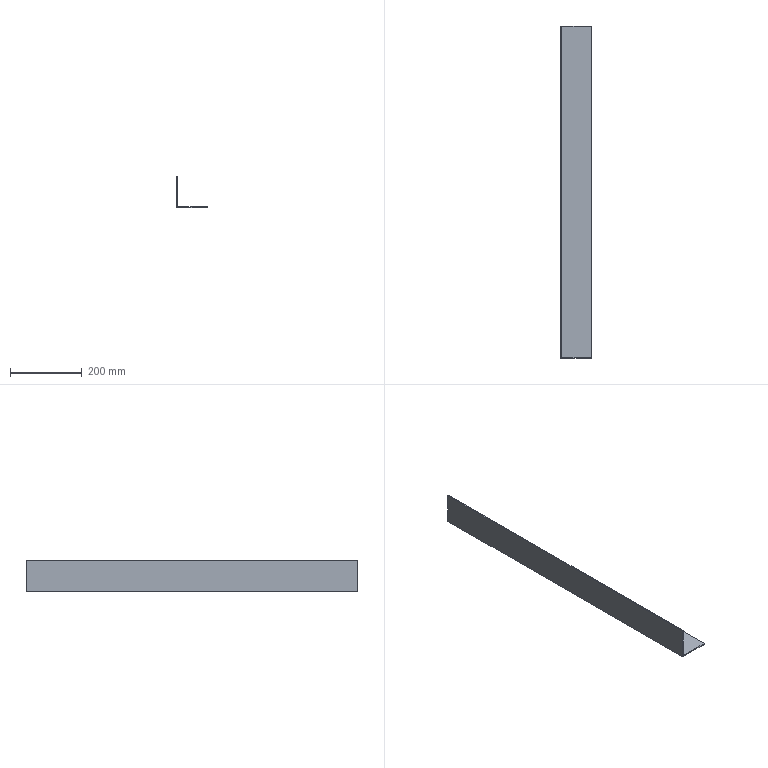Part | NX | features DATUM_CSYS 1, EXTRUDE 1, LINKED_CURVE 1, MOVE_FACE 1 | 1 solid | 8 faces | box 85 x 926 x 88 mm | volume 472260 mm3 | plane 8
STEP:
#1=CARTESIAN_POINT('',(-543.,-463.,-91.163));
#2=VERTEX_POINT('',#1);
#3=CARTESIAN_POINT('',(-543.,-463.,-3.163));
#4=VERTEX_POINT('',#3);
#5=CARTESIAN_POINT('',(-543.,-463.,-88.163));
#6=DIRECTION('',(0.,0.,1.));
#7=VECTOR('',#6,1000.);
#8=LINE('',#5,#7);
#9=EDGE_CURVE('',#2,#4,#8,.T.);
#10=ORIENTED_EDGE('',*,*,#9,.F.);
#11=CARTESIAN_POINT('',(-458.,-463.,-91.163));
#12=VERTEX_POINT('',#11);
#13=CARTESIAN_POINT('',(-455.,-463.,-91.163));
#14=DIRECTION('',(-1.,0.,0.));
#15=VECTOR('',#14,1000.);
#16=LINE('',#13,#15);
#17=EDGE_CURVE('',#12,#2,#16,.T.);
#18=ORIENTED_EDGE('',*,*,#17,.F.);
#19=CARTESIAN_POINT('',(-458.,-463.,-88.163));
#20=VERTEX_POINT('',#19);
#21=CARTESIAN_POINT('',(-458.,-463.,-88.163));
#22=DIRECTION('',(0.,0.,-1.));
#23=VECTOR('',#22,1000.);
#24=LINE('',#21,#23);
#25=EDGE_CURVE('',#20,#12,#24,.T.);
#26=ORIENTED_EDGE('',*,*,#25,.F.);
#27=CARTESIAN_POINT('',(-540.,-463.,-88.163));
#28=VERTEX_POINT('',#27);
#29=CARTESIAN_POINT('',(-455.,-463.,-88.163));
#30=DIRECTION('',(-1.,0.,0.));
#31=VECTOR('',#30,1000.);
#32=LINE('',#29,#31);
#33=EDGE_CURVE('',#20,#28,#32,.T.);
#34=ORIENTED_EDGE('',*,*,#33,.T.);
#35=CARTESIAN_POINT('',(-540.,-463.,-3.163));
#36=VERTEX_POINT('',#35);
#37=CARTESIAN_POINT('',(-540.,-463.,-88.163));
#38=DIRECTION('',(0.,0.,1.));
#39=VECTOR('',#38,1000.);
#40=LINE('',#37,#39);
#41=EDGE_CURVE('',#28,#36,#40,.T.);
#42=ORIENTED_EDGE('',*,*,#41,.T.);
#43=CARTESIAN_POINT('',(-540.,-463.,-3.163));
#44=DIRECTION('',(-1.,0.,0.));
#45=VECTOR('',#44,1000.);
#46=LINE('',#43,#45);
#47=EDGE_CURVE('',#36,#4,#46,.T.);
#48=ORIENTED_EDGE('',*,*,#47,.T.);
#49=EDGE_LOOP('',(#10,#18,#26,#34,#42,#48));
#50=FACE_BOUND('',#49,.T.);
#51=CARTESIAN_POINT('',(-540.,-463.,-88.163));
#52=DIRECTION('',(0.,-1.,0.));
#53=DIRECTION('',(0.,0.,1.));
#54=AXIS2_PLACEMENT_3D('',#51,#52,#53);
#55=PLANE('',#54);
#56=ADVANCED_FACE('',(#50),#55,.T.);
#57=ORIENTED_EDGE('',*,*,#47,.F.);
#58=CARTESIAN_POINT('',(-540.,463.,-3.163));
#59=VERTEX_POINT('',#58);
#60=CARTESIAN_POINT('',(-540.,-463.,-3.163));
#61=DIRECTION('',(0.,1.,0.));
#62=VECTOR('',#61,1000.);
#63=LINE('',#60,#62);
#64=EDGE_CURVE('',#36,#59,#63,.T.);
#65=ORIENTED_EDGE('',*,*,#64,.T.);
#66=CARTESIAN_POINT('',(-543.,463.,-3.163));
#67=VERTEX_POINT('',#66);
#68=CARTESIAN_POINT('',(-540.,463.,-3.163));
#69=DIRECTION('',(-1.,0.,0.));
#70=VECTOR('',#69,1000.);
#71=LINE('',#68,#70);
#72=EDGE_CURVE('',#59,#67,#71,.T.);
#73=ORIENTED_EDGE('',*,*,#72,.T.);
#74=CARTESIAN_POINT('',(-543.,-463.,-3.163));
#75=DIRECTION('',(0.,1.,0.));
#76=VECTOR('',#75,1000.);
#77=LINE('',#74,#76);
#78=EDGE_CURVE('',#4,#67,#77,.T.);
#79=ORIENTED_EDGE('',*,*,#78,.F.);
#80=EDGE_LOOP('',(#57,#65,#73,#79));
#81=FACE_BOUND('',#80,.T.);
#82=CARTESIAN_POINT('',(-540.,-463.,-3.163));
#83=DIRECTION('',(0.,0.,1.));
#84=DIRECTION('',(0.,1.,0.));
#85=AXIS2_PLACEMENT_3D('',#82,#83,#84);
#86=PLANE('',#85);
#87=ADVANCED_FACE('',(#81),#86,.T.);
#88=CARTESIAN_POINT('',(-458.,463.,-91.163));
#89=VERTEX_POINT('',#88);
#90=CARTESIAN_POINT('',(-543.,463.,-91.163));
#91=VERTEX_POINT('',#90);
#92=CARTESIAN_POINT('',(-455.,463.,-91.163));
#93=DIRECTION('',(-1.,0.,0.));
#94=VECTOR('',#93,1000.);
#95=LINE('',#92,#94);
#96=EDGE_CURVE('',#89,#91,#95,.T.);
#97=ORIENTED_EDGE('',*,*,#96,.T.);
#98=CARTESIAN_POINT('',(-543.,463.,-88.163));
#99=DIRECTION('',(0.,0.,1.));
#100=VECTOR('',#99,1000.);
#101=LINE('',#98,#100);
#102=EDGE_CURVE('',#91,#67,#101,.T.);
#103=ORIENTED_EDGE('',*,*,#102,.T.);
#104=ORIENTED_EDGE('',*,*,#72,.F.);
#105=CARTESIAN_POINT('',(-540.,463.,-88.163));
#106=VERTEX_POINT('',#105);
#107=CARTESIAN_POINT('',(-540.,463.,-88.163));
#108=DIRECTION('',(0.,0.,1.));
#109=VECTOR('',#108,1000.);
#110=LINE('',#107,#109);
#111=EDGE_CURVE('',#106,#59,#110,.T.);
#112=ORIENTED_EDGE('',*,*,#111,.F.);
#113=CARTESIAN_POINT('',(-458.,463.,-88.163));
#114=VERTEX_POINT('',#113);
#115=CARTESIAN_POINT('',(-455.,463.,-88.163));
#116=DIRECTION('',(-1.,0.,0.));
#117=VECTOR('',#116,1000.);
#118=LINE('',#115,#117);
#119=EDGE_CURVE('',#114,#106,#118,.T.);
#120=ORIENTED_EDGE('',*,*,#119,.F.);
#121=CARTESIAN_POINT('',(-458.,463.,-88.163));
#122=DIRECTION('',(0.,0.,-1.));
#123=VECTOR('',#122,1000.);
#124=LINE('',#121,#123);
#125=EDGE_CURVE('',#114,#89,#124,.T.);
#126=ORIENTED_EDGE('',*,*,#125,.T.);
#127=EDGE_LOOP('',(#97,#103,#104,#112,#120,#126));
#128=FACE_BOUND('',#127,.T.);
#129=CARTESIAN_POINT('',(-455.,463.,-88.163));
#130=DIRECTION('',(0.,-1.,0.));
#131=DIRECTION('',(-1.,0.,0.));
#132=AXIS2_PLACEMENT_3D('',#129,#130,#131);
#133=PLANE('',#132);
#134=ADVANCED_FACE('',(#128),#133,.F.);
#135=CARTESIAN_POINT('',(-458.,-463.,-88.163));
#136=DIRECTION('',(0.,1.,0.));
#137=VECTOR('',#136,1000.);
#138=LINE('',#135,#137);
#139=EDGE_CURVE('',#20,#114,#138,.T.);
#140=ORIENTED_EDGE('',*,*,#139,.F.);
#141=ORIENTED_EDGE('',*,*,#25,.T.);
#142=CARTESIAN_POINT('',(-458.,-463.,-91.163));
#143=DIRECTION('',(0.,1.,0.));
#144=VECTOR('',#143,1000.);
#145=LINE('',#142,#144);
#146=EDGE_CURVE('',#12,#89,#145,.T.);
#147=ORIENTED_EDGE('',*,*,#146,.T.);
#148=ORIENTED_EDGE('',*,*,#125,.F.);
#149=EDGE_LOOP('',(#140,#141,#147,#148));
#150=FACE_BOUND('',#149,.T.);
#151=CARTESIAN_POINT('',(-458.,-463.,-88.163));
#152=DIRECTION('',(-1.,0.,0.));
#153=DIRECTION('',(0.,1.,0.));
#154=AXIS2_PLACEMENT_3D('',#151,#152,#153);
#155=PLANE('',#154);
#156=ADVANCED_FACE('',(#150),#155,.F.);
#157=ORIENTED_EDGE('',*,*,#96,.F.);
#158=ORIENTED_EDGE('',*,*,#146,.F.);
#159=ORIENTED_EDGE('',*,*,#17,.T.);
#160=CARTESIAN_POINT('',(-543.,-463.,-91.163));
#161=DIRECTION('',(0.,1.,0.));
#162=VECTOR('',#161,1000.);
#163=LINE('',#160,#162);
#164=EDGE_CURVE('',#2,#91,#163,.T.);
#165=ORIENTED_EDGE('',*,*,#164,.T.);
#166=EDGE_LOOP('',(#157,#158,#159,#165));
#167=FACE_BOUND('',#166,.T.);
#168=CARTESIAN_POINT('',(-455.,-463.,-91.163));
#169=DIRECTION('',(0.,0.,-1.));
#170=DIRECTION('',(-1.,0.,0.));
#171=AXIS2_PLACEMENT_3D('',#168,#169,#170);
#172=PLANE('',#171);
#173=ADVANCED_FACE('',(#167),#172,.T.);
#174=ORIENTED_EDGE('',*,*,#102,.F.);
#175=ORIENTED_EDGE('',*,*,#164,.F.);
#176=ORIENTED_EDGE('',*,*,#9,.T.);
#177=ORIENTED_EDGE('',*,*,#78,.T.);
#178=EDGE_LOOP('',(#174,#175,#176,#177));
#179=FACE_BOUND('',#178,.T.);
#180=CARTESIAN_POINT('',(-543.,-463.,-88.163));
#181=DIRECTION('',(-1.,0.,0.));
#182=DIRECTION('',(0.,0.,1.));
#183=AXIS2_PLACEMENT_3D('',#180,#181,#182);
#184=PLANE('',#183);
#185=ADVANCED_FACE('',(#179),#184,.T.);
#186=ORIENTED_EDGE('',*,*,#119,.T.);
#187=CARTESIAN_POINT('',(-540.,-463.,-88.163));
#188=DIRECTION('',(0.,1.,0.));
#189=VECTOR('',#188,1000.);
#190=LINE('',#187,#189);
#191=EDGE_CURVE('',#28,#106,#190,.T.);
#192=ORIENTED_EDGE('',*,*,#191,.F.);
#193=ORIENTED_EDGE('',*,*,#33,.F.);
#194=ORIENTED_EDGE('',*,*,#139,.T.);
#195=EDGE_LOOP('',(#186,#192,#193,#194));
#196=FACE_BOUND('',#195,.T.);
#197=CARTESIAN_POINT('',(-455.,-463.,-88.163));
#198=DIRECTION('',(0.,0.,-1.));
#199=DIRECTION('',(-1.,0.,0.));
#200=AXIS2_PLACEMENT_3D('',#197,#198,#199);
#201=PLANE('',#200);
#202=ADVANCED_FACE('',(#196),#201,.F.);
#203=ORIENTED_EDGE('',*,*,#111,.T.);
#204=ORIENTED_EDGE('',*,*,#64,.F.);
#205=ORIENTED_EDGE('',*,*,#41,.F.);
#206=ORIENTED_EDGE('',*,*,#191,.T.);
#207=EDGE_LOOP('',(#203,#204,#205,#206));
#208=FACE_BOUND('',#207,.T.);
#209=CARTESIAN_POINT('',(-540.,-463.,-88.163));
#210=DIRECTION('',(-1.,0.,0.));
#211=DIRECTION('',(0.,0.,1.));
#212=AXIS2_PLACEMENT_3D('',#209,#210,#211);
#213=PLANE('',#212);
#214=ADVANCED_FACE('',(#208),#213,.F.);
#215=CLOSED_SHELL('',(#56,#87,#134,#156,#173,#185,#202,#214));
#216=MANIFOLD_SOLID_BREP('',#215);
#217=(LENGTH_UNIT()NAMED_UNIT(*)SI_UNIT(.MILLI.,.METRE.));
#218=UNCERTAINTY_MEASURE_WITH_UNIT(LENGTH_MEASURE(0.00001),#217,'','');
#219=(NAMED_UNIT(*)PLANE_ANGLE_UNIT()SI_UNIT($,.RADIAN.));
#220=(NAMED_UNIT(*)SI_UNIT($,.STERADIAN.)SOLID_ANGLE_UNIT());
#221=(GEOMETRIC_REPRESENTATION_CONTEXT(3)GLOBAL_UNCERTAINTY_ASSIGNED_CONTEXT((#218))GLOBAL_UNIT_ASSIGNED_CONTEXT((#217,#219,#220))REPRESENTATION_CONTEXT('',''));
#222=ADVANCED_BREP_SHAPE_REPRESENTATION('',(#216),#221);